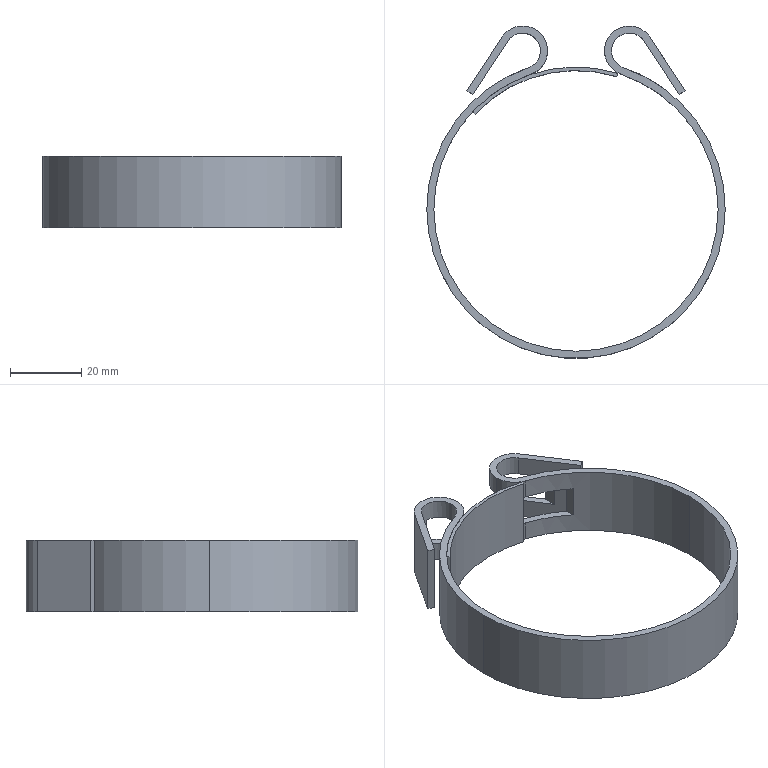Part | SolidWorks | features ICE 3, Extrusion 1 | 2 solids | 38 faces | box 84 x 93.542 x 20 mm | volume 12226 mm3 | plane 20 | cylinder 18 | commonest cylinder face diameters 10 x5 14 x5 80 x4 84 x3 78 x1
STEP:
#1=CARTESIAN_POINT('',(12.766,37.908,5.5));
#2=VERTEX_POINT('',#1);
#3=CARTESIAN_POINT('',(8.,44.542,5.5));
#4=VERTEX_POINT('',#3);
#5=CARTESIAN_POINT('',(15.,44.542,5.5));
#6=DIRECTION('',(0.,0.,-1.));
#7=DIRECTION('',(-1.,0.,0.));
#8=AXIS2_PLACEMENT_3D('',#5,#6,#7);
#9=CIRCLE('',#8,7.);
#10=EDGE_CURVE('',#2,#4,#9,.T.);
#11=ORIENTED_EDGE('',*,*,#10,.T.);
#12=CARTESIAN_POINT('',(8.,44.542,0.));
#13=VERTEX_POINT('',#12);
#14=CARTESIAN_POINT('',(8.,44.542,20.));
#15=DIRECTION('',(0.,0.,-1.));
#16=VECTOR('',#15,1000.);
#17=LINE('',#14,#16);
#18=EDGE_CURVE('',#4,#13,#17,.T.);
#19=ORIENTED_EDGE('',*,*,#18,.T.);
#20=CARTESIAN_POINT('',(12.766,37.908,0.));
#21=VERTEX_POINT('',#20);
#22=CARTESIAN_POINT('',(15.,44.542,0.));
#23=DIRECTION('',(0.,0.,1.));
#24=DIRECTION('',(-1.,0.,0.));
#25=AXIS2_PLACEMENT_3D('',#22,#23,#24);
#26=CIRCLE('',#25,7.);
#27=EDGE_CURVE('',#13,#21,#26,.T.);
#28=ORIENTED_EDGE('',*,*,#27,.T.);
#29=CARTESIAN_POINT('',(12.766,37.908,20.));
#30=DIRECTION('',(0.,0.,-1.));
#31=VECTOR('',#30,1000.);
#32=LINE('',#29,#31);
#33=EDGE_CURVE('',#2,#21,#32,.T.);
#34=ORIENTED_EDGE('',*,*,#33,.F.);
#35=EDGE_LOOP('',(#11,#19,#28,#34));
#36=FACE_OUTER_BOUND('',#35,.T.);
#37=CARTESIAN_POINT('',(15.,44.542,20.));
#38=DIRECTION('',(0.,0.,-1.));
#39=DIRECTION('',(-1.,0.,0.));
#40=AXIS2_PLACEMENT_3D('',#37,#38,#39);
#41=CYLINDRICAL_SURFACE('',#40,7.);
#42=ADVANCED_FACE('',(#36),#41,.T.);
#43=CARTESIAN_POINT('',(10.,44.542,20.));
#44=VERTEX_POINT('',#43);
#45=CARTESIAN_POINT('',(19.178,47.288,20.));
#46=VERTEX_POINT('',#45);
#47=CARTESIAN_POINT('',(15.,44.542,20.));
#48=DIRECTION('',(0.,0.,-1.));
#49=DIRECTION('',(-1.,0.,0.));
#50=AXIS2_PLACEMENT_3D('',#47,#48,#49);
#51=CIRCLE('',#50,5.);
#52=EDGE_CURVE('',#44,#46,#51,.T.);
#53=ORIENTED_EDGE('',*,*,#52,.F.);
#54=CARTESIAN_POINT('',(10.,44.542,14.5));
#55=VERTEX_POINT('',#54);
#56=CARTESIAN_POINT('',(10.,44.542,20.));
#57=DIRECTION('',(0.,0.,-1.));
#58=VECTOR('',#57,1000.);
#59=LINE('',#56,#58);
#60=EDGE_CURVE('',#44,#55,#59,.T.);
#61=ORIENTED_EDGE('',*,*,#60,.T.);
#62=CARTESIAN_POINT('',(19.178,47.288,14.5));
#63=VERTEX_POINT('',#62);
#64=CARTESIAN_POINT('',(15.,44.542,14.5));
#65=DIRECTION('',(0.,0.,-1.));
#66=DIRECTION('',(1.,0.,0.));
#67=AXIS2_PLACEMENT_3D('',#64,#65,#66);
#68=CIRCLE('',#67,5.);
#69=EDGE_CURVE('',#55,#63,#68,.T.);
#70=ORIENTED_EDGE('',*,*,#69,.T.);
#71=CARTESIAN_POINT('',(19.178,47.288,20.));
#72=DIRECTION('',(0.,0.,-1.));
#73=VECTOR('',#72,1000.);
#74=LINE('',#71,#73);
#75=EDGE_CURVE('',#46,#63,#74,.T.);
#76=ORIENTED_EDGE('',*,*,#75,.F.);
#77=EDGE_LOOP('',(#53,#61,#70,#76));
#78=FACE_OUTER_BOUND('',#77,.T.);
#79=CARTESIAN_POINT('',(15.,44.542,20.));
#80=DIRECTION('',(0.,0.,-1.));
#81=DIRECTION('',(-1.,0.,0.));
#82=AXIS2_PLACEMENT_3D('',#79,#80,#81);
#83=CYLINDRICAL_SURFACE('',#82,5.);
#84=ADVANCED_FACE('',(#78),#83,.F.);
#85=CARTESIAN_POINT('',(40.,0.,20.));
#86=VERTEX_POINT('',#85);
#87=CARTESIAN_POINT('',(-40.,0.,20.));
#88=VERTEX_POINT('',#87);
#89=CARTESIAN_POINT('',(0.,0.,20.));
#90=DIRECTION('',(0.,0.,-1.));
#91=DIRECTION('',(1.,0.,0.));
#92=AXIS2_PLACEMENT_3D('',#89,#90,#91);
#93=CIRCLE('',#92,40.);
#94=EDGE_CURVE('',#86,#88,#93,.T.);
#95=ORIENTED_EDGE('',*,*,#94,.F.);
#96=CARTESIAN_POINT('',(40.,0.,0.));
#97=VERTEX_POINT('',#96);
#98=CARTESIAN_POINT('',(40.,0.,20.));
#99=DIRECTION('',(0.,0.,-1.));
#100=VECTOR('',#99,1000.);
#101=LINE('',#98,#100);
#102=EDGE_CURVE('',#86,#97,#101,.T.);
#103=ORIENTED_EDGE('',*,*,#102,.T.);
#104=CARTESIAN_POINT('',(-40.,0.,0.));
#105=VERTEX_POINT('',#104);
#106=CARTESIAN_POINT('',(0.,0.,0.));
#107=DIRECTION('',(0.,0.,-1.));
#108=DIRECTION('',(1.,0.,0.));
#109=AXIS2_PLACEMENT_3D('',#106,#107,#108);
#110=CIRCLE('',#109,40.);
#111=EDGE_CURVE('',#97,#105,#110,.T.);
#112=ORIENTED_EDGE('',*,*,#111,.T.);
#113=CARTESIAN_POINT('',(-40.,0.,20.));
#114=DIRECTION('',(0.,0.,-1.));
#115=VECTOR('',#114,1000.);
#116=LINE('',#113,#115);
#117=EDGE_CURVE('',#88,#105,#116,.T.);
#118=ORIENTED_EDGE('',*,*,#117,.F.);
#119=EDGE_LOOP('',(#95,#103,#112,#118));
#120=FACE_OUTER_BOUND('',#119,.T.);
#121=CARTESIAN_POINT('',(0.,0.,20.));
#122=DIRECTION('',(0.,0.,-1.));
#123=DIRECTION('',(-1.,0.,0.));
#124=AXIS2_PLACEMENT_3D('',#121,#122,#123);
#125=CYLINDRICAL_SURFACE('',#124,40.);
#126=ADVANCED_FACE('',(#120),#125,.F.);
#127=CARTESIAN_POINT('',(-12.766,37.908,20.));
#128=VERTEX_POINT('',#127);
#129=CARTESIAN_POINT('',(0.,0.,20.));
#130=DIRECTION('',(0.,0.,-1.));
#131=DIRECTION('',(1.,0.,0.));
#132=AXIS2_PLACEMENT_3D('',#129,#130,#131);
#133=CIRCLE('',#132,40.);
#134=EDGE_CURVE('',#88,#128,#133,.T.);
#135=ORIENTED_EDGE('',*,*,#134,.F.);
#136=ORIENTED_EDGE('',*,*,#117,.T.);
#137=CARTESIAN_POINT('',(-12.766,37.908,0.));
#138=VERTEX_POINT('',#137);
#139=CARTESIAN_POINT('',(0.,0.,0.));
#140=DIRECTION('',(0.,0.,-1.));
#141=DIRECTION('',(1.,0.,0.));
#142=AXIS2_PLACEMENT_3D('',#139,#140,#141);
#143=CIRCLE('',#142,40.);
#144=EDGE_CURVE('',#105,#138,#143,.T.);
#145=ORIENTED_EDGE('',*,*,#144,.T.);
#146=CARTESIAN_POINT('',(-12.766,37.908,5.5));
#147=VERTEX_POINT('',#146);
#148=CARTESIAN_POINT('',(-12.766,37.908,20.));
#149=DIRECTION('',(0.,0.,-1.));
#150=VECTOR('',#149,1000.);
#151=LINE('',#148,#150);
#152=EDGE_CURVE('',#147,#138,#151,.T.);
#153=ORIENTED_EDGE('',*,*,#152,.F.);
#154=CARTESIAN_POINT('',(-15.,37.081,5.5));
#155=VERTEX_POINT('',#154);
#156=CARTESIAN_POINT('',(0.,0.,5.5));
#157=DIRECTION('',(0.,0.,-1.));
#158=DIRECTION('',(1.,0.,0.));
#159=AXIS2_PLACEMENT_3D('',#156,#157,#158);
#160=CIRCLE('',#159,40.);
#161=EDGE_CURVE('',#155,#147,#160,.T.);
#162=ORIENTED_EDGE('',*,*,#161,.F.);
#163=CARTESIAN_POINT('',(-15.,37.081,14.5));
#164=VERTEX_POINT('',#163);
#165=CARTESIAN_POINT('',(-15.,37.081,20.));
#166=DIRECTION('',(0.,0.,-1.));
#167=VECTOR('',#166,1000.);
#168=LINE('',#165,#167);
#169=EDGE_CURVE('',#164,#155,#168,.T.);
#170=ORIENTED_EDGE('',*,*,#169,.F.);
#171=CARTESIAN_POINT('',(-12.766,37.908,14.5));
#172=VERTEX_POINT('',#171);
#173=CARTESIAN_POINT('',(0.,0.,14.5));
#174=DIRECTION('',(0.,0.,1.));
#175=DIRECTION('',(-1.,0.,0.));
#176=AXIS2_PLACEMENT_3D('',#173,#174,#175);
#177=CIRCLE('',#176,40.);
#178=EDGE_CURVE('',#172,#164,#177,.T.);
#179=ORIENTED_EDGE('',*,*,#178,.F.);
#180=CARTESIAN_POINT('',(-12.766,37.908,20.));
#181=DIRECTION('',(0.,0.,-1.));
#182=VECTOR('',#181,1000.);
#183=LINE('',#180,#182);
#184=EDGE_CURVE('',#128,#172,#183,.T.);
#185=ORIENTED_EDGE('',*,*,#184,.F.);
#186=EDGE_LOOP('',(#135,#136,#145,#153,#162,#170,#179,#185));
#187=FACE_OUTER_BOUND('',#186,.T.);
#188=CARTESIAN_POINT('',(0.,0.,20.));
#189=DIRECTION('',(0.,0.,-1.));
#190=DIRECTION('',(-1.,0.,0.));
#191=AXIS2_PLACEMENT_3D('',#188,#189,#190);
#192=CYLINDRICAL_SURFACE('',#191,40.);
#193=ADVANCED_FACE('',(#187),#192,.F.);
#194=CARTESIAN_POINT('',(42.,0.,20.));
#195=VERTEX_POINT('',#194);
#196=CARTESIAN_POINT('',(13.404,39.804,20.));
#197=VERTEX_POINT('',#196);
#198=CARTESIAN_POINT('',(0.,0.,20.));
#199=DIRECTION('',(0.,0.,1.));
#200=DIRECTION('',(1.,0.,0.));
#201=AXIS2_PLACEMENT_3D('',#198,#199,#200);
#202=CIRCLE('',#201,42.);
#203=EDGE_CURVE('',#195,#197,#202,.T.);
#204=ORIENTED_EDGE('',*,*,#203,.F.);
#205=CARTESIAN_POINT('',(42.,0.,0.));
#206=VERTEX_POINT('',#205);
#207=CARTESIAN_POINT('',(42.,0.,20.));
#208=DIRECTION('',(0.,0.,-1.));
#209=VECTOR('',#208,1000.);
#210=LINE('',#207,#209);
#211=EDGE_CURVE('',#195,#206,#210,.T.);
#212=ORIENTED_EDGE('',*,*,#211,.T.);
#213=CARTESIAN_POINT('',(13.404,39.804,0.));
#214=VERTEX_POINT('',#213);
#215=CARTESIAN_POINT('',(0.,0.,0.));
#216=DIRECTION('',(0.,0.,1.));
#217=DIRECTION('',(1.,0.,0.));
#218=AXIS2_PLACEMENT_3D('',#215,#216,#217);
#219=CIRCLE('',#218,42.);
#220=EDGE_CURVE('',#206,#214,#219,.T.);
#221=ORIENTED_EDGE('',*,*,#220,.T.);
#222=CARTESIAN_POINT('',(13.404,39.804,5.5));
#223=VERTEX_POINT('',#222);
#224=CARTESIAN_POINT('',(13.404,39.804,20.));
#225=DIRECTION('',(0.,0.,-1.));
#226=VECTOR('',#225,1000.);
#227=LINE('',#224,#226);
#228=EDGE_CURVE('',#223,#214,#227,.T.);
#229=ORIENTED_EDGE('',*,*,#228,.F.);
#230=CARTESIAN_POINT('',(25.,33.749,5.5));
#231=VERTEX_POINT('',#230);
#232=CARTESIAN_POINT('',(0.,0.,5.5));
#233=DIRECTION('',(0.,0.,-1.));
#234=DIRECTION('',(-1.,0.,0.));
#235=AXIS2_PLACEMENT_3D('',#232,#233,#234);
#236=CIRCLE('',#235,42.);
#237=EDGE_CURVE('',#223,#231,#236,.T.);
#238=ORIENTED_EDGE('',*,*,#237,.T.);
#239=CARTESIAN_POINT('',(25.,33.749,14.5));
#240=VERTEX_POINT('',#239);
#241=CARTESIAN_POINT('',(25.,33.749,20.));
#242=DIRECTION('',(0.,0.,1.));
#243=VECTOR('',#242,1000.);
#244=LINE('',#241,#243);
#245=EDGE_CURVE('',#231,#240,#244,.T.);
#246=ORIENTED_EDGE('',*,*,#245,.T.);
#247=CARTESIAN_POINT('',(13.404,39.804,14.5));
#248=VERTEX_POINT('',#247);
#249=CARTESIAN_POINT('',(0.,0.,14.5));
#250=DIRECTION('',(0.,0.,1.));
#251=DIRECTION('',(1.,0.,0.));
#252=AXIS2_PLACEMENT_3D('',#249,#250,#251);
#253=CIRCLE('',#252,42.);
#254=EDGE_CURVE('',#240,#248,#253,.T.);
#255=ORIENTED_EDGE('',*,*,#254,.T.);
#256=CARTESIAN_POINT('',(13.404,39.804,20.));
#257=DIRECTION('',(0.,0.,-1.));
#258=VECTOR('',#257,1000.);
#259=LINE('',#256,#258);
#260=EDGE_CURVE('',#197,#248,#259,.T.);
#261=ORIENTED_EDGE('',*,*,#260,.F.);
#262=EDGE_LOOP('',(#204,#212,#221,#229,#238,#246,#255,#261));
#263=FACE_OUTER_BOUND('',#262,.T.);
#264=CARTESIAN_POINT('',(0.,0.,20.));
#265=DIRECTION('',(0.,0.,-1.));
#266=DIRECTION('',(-1.,0.,0.));
#267=AXIS2_PLACEMENT_3D('',#264,#265,#266);
#268=CYLINDRICAL_SURFACE('',#267,42.);
#269=ADVANCED_FACE('',(#263),#268,.T.);
#270=ORIENTED_EDGE('',*,*,#211,.F.);
#271=CARTESIAN_POINT('',(-42.,0.,20.));
#272=VERTEX_POINT('',#271);
#273=CARTESIAN_POINT('',(0.,0.,20.));
#274=DIRECTION('',(0.,0.,1.));
#275=DIRECTION('',(1.,0.,0.));
#276=AXIS2_PLACEMENT_3D('',#273,#274,#275);
#277=CIRCLE('',#276,42.);
#278=EDGE_CURVE('',#272,#195,#277,.T.);
#279=ORIENTED_EDGE('',*,*,#278,.F.);
#280=CARTESIAN_POINT('',(-42.,0.,0.));
#281=VERTEX_POINT('',#280);
#282=CARTESIAN_POINT('',(-42.,0.,20.));
#283=DIRECTION('',(0.,0.,-1.));
#284=VECTOR('',#283,1000.);
#285=LINE('',#282,#284);
#286=EDGE_CURVE('',#272,#281,#285,.T.);
#287=ORIENTED_EDGE('',*,*,#286,.T.);
#288=CARTESIAN_POINT('',(0.,0.,0.));
#289=DIRECTION('',(0.,0.,1.));
#290=DIRECTION('',(1.,0.,0.));
#291=AXIS2_PLACEMENT_3D('',#288,#289,#290);
#292=CIRCLE('',#291,42.);
#293=EDGE_CURVE('',#281,#206,#292,.T.);
#294=ORIENTED_EDGE('',*,*,#293,.T.);
#295=EDGE_LOOP('',(#270,#279,#287,#294));
#296=FACE_OUTER_BOUND('',#295,.T.);
#297=CARTESIAN_POINT('',(0.,0.,20.));
#298=DIRECTION('',(0.,0.,-1.));
#299=DIRECTION('',(-1.,0.,0.));
#300=AXIS2_PLACEMENT_3D('',#297,#298,#299);
#301=CYLINDRICAL_SURFACE('',#300,42.);
#302=ADVANCED_FACE('',(#296),#301,.T.);
#303=CARTESIAN_POINT('',(8.,44.542,20.));
#304=VERTEX_POINT('',#303);
#305=CARTESIAN_POINT('',(12.766,37.908,20.));
#306=VERTEX_POINT('',#305);
#307=CARTESIAN_POINT('',(15.,44.542,20.));
#308=DIRECTION('',(0.,0.,1.));
#309=DIRECTION('',(-1.,0.,0.));
#310=AXIS2_PLACEMENT_3D('',#307,#308,#309);
#311=CIRCLE('',#310,7.);
#312=EDGE_CURVE('',#304,#306,#311,.T.);
#313=ORIENTED_EDGE('',*,*,#312,.F.);
#314=CARTESIAN_POINT('',(8.,44.542,14.5));
#315=VERTEX_POINT('',#314);
#316=CARTESIAN_POINT('',(8.,44.542,20.));
#317=DIRECTION('',(0.,0.,-1.));
#318=VECTOR('',#317,1000.);
#319=LINE('',#316,#318);
#320=EDGE_CURVE('',#304,#315,#319,.T.);
#321=ORIENTED_EDGE('',*,*,#320,.T.);
#322=CARTESIAN_POINT('',(12.766,37.908,14.5));
#323=VERTEX_POINT('',#322);
#324=CARTESIAN_POINT('',(15.,44.542,14.5));
#325=DIRECTION('',(0.,0.,1.));
#326=DIRECTION('',(1.,0.,0.));
#327=AXIS2_PLACEMENT_3D('',#324,#325,#326);
#328=CIRCLE('',#327,7.);
#329=EDGE_CURVE('',#315,#323,#328,.T.);
#330=ORIENTED_EDGE('',*,*,#329,.T.);
#331=CARTESIAN_POINT('',(12.766,37.908,20.));
#332=DIRECTION('',(0.,0.,-1.));
#333=VECTOR('',#332,1000.);
#334=LINE('',#331,#333);
#335=EDGE_CURVE('',#306,#323,#334,.T.);
#336=ORIENTED_EDGE('',*,*,#335,.F.);
#337=EDGE_LOOP('',(#313,#321,#330,#336));
#338=FACE_OUTER_BOUND('',#337,.T.);
#339=CARTESIAN_POINT('',(15.,44.542,20.));
#340=DIRECTION('',(0.,0.,-1.));
#341=DIRECTION('',(-1.,0.,0.));
#342=AXIS2_PLACEMENT_3D('',#339,#340,#341);
#343=CYLINDRICAL_SURFACE('',#342,7.);
#344=ADVANCED_FACE('',(#338),#343,.T.);
#345=CARTESIAN_POINT('',(19.178,47.288,5.5));
#346=VERTEX_POINT('',#345);
#347=CARTESIAN_POINT('',(10.,44.542,5.5));
#348=VERTEX_POINT('',#347);
#349=CARTESIAN_POINT('',(15.,44.542,5.5));
#350=DIRECTION('',(0.,0.,1.));
#351=DIRECTION('',(-1.,0.,0.));
#352=AXIS2_PLACEMENT_3D('',#349,#350,#351);
#353=CIRCLE('',#352,5.);
#354=EDGE_CURVE('',#346,#348,#353,.T.);
#355=ORIENTED_EDGE('',*,*,#354,.T.);
#356=CARTESIAN_POINT('',(10.,44.542,0.));
#357=VERTEX_POINT('',#356);
#358=CARTESIAN_POINT('',(10.,44.542,20.));
#359=DIRECTION('',(0.,0.,-1.));
#360=VECTOR('',#359,1000.);
#361=LINE('',#358,#360);
#362=EDGE_CURVE('',#348,#357,#361,.T.);
#363=ORIENTED_EDGE('',*,*,#362,.T.);
#364=CARTESIAN_POINT('',(19.178,47.288,0.));
#365=VERTEX_POINT('',#364);
#366=CARTESIAN_POINT('',(15.,44.542,0.));
#367=DIRECTION('',(0.,0.,-1.));
#368=DIRECTION('',(-1.,0.,0.));
#369=AXIS2_PLACEMENT_3D('',#366,#367,#368);
#370=CIRCLE('',#369,5.);
#371=EDGE_CURVE('',#357,#365,#370,.T.);
#372=ORIENTED_EDGE('',*,*,#371,.T.);
#373=CARTESIAN_POINT('',(19.178,47.288,20.));
#374=DIRECTION('',(0.,0.,-1.));
#375=VECTOR('',#374,1000.);
#376=LINE('',#373,#375);
#377=EDGE_CURVE('',#346,#365,#376,.T.);
#378=ORIENTED_EDGE('',*,*,#377,.F.);
#379=EDGE_LOOP('',(#355,#363,#372,#378));
#380=FACE_OUTER_BOUND('',#379,.T.);
#381=CARTESIAN_POINT('',(15.,44.542,20.));
#382=DIRECTION('',(0.,0.,-1.));
#383=DIRECTION('',(-1.,0.,0.));
#384=AXIS2_PLACEMENT_3D('',#381,#382,#383);
#385=CYLINDRICAL_SURFACE('',#384,5.);
#386=ADVANCED_FACE('',(#380),#385,.F.);
#387=ORIENTED_EDGE('',*,*,#362,.F.);
#388=CARTESIAN_POINT('',(15.,44.542,5.5));
#389=DIRECTION('',(0.,0.,1.));
#390=DIRECTION('',(-1.,0.,0.));
#391=AXIS2_PLACEMENT_3D('',#388,#389,#390);
#392=CIRCLE('',#391,5.);
#393=EDGE_CURVE('',#348,#223,#392,.T.);
#394=ORIENTED_EDGE('',*,*,#393,.T.);
#395=ORIENTED_EDGE('',*,*,#228,.T.);
#396=CARTESIAN_POINT('',(15.,44.542,0.));
#397=DIRECTION('',(0.,0.,-1.));
#398=DIRECTION('',(-1.,0.,0.));
#399=AXIS2_PLACEMENT_3D('',#396,#397,#398);
#400=CIRCLE('',#399,5.);
#401=EDGE_CURVE('',#214,#357,#400,.T.);
#402=ORIENTED_EDGE('',*,*,#401,.T.);
#403=EDGE_LOOP('',(#387,#394,#395,#402));
#404=FACE_OUTER_BOUND('',#403,.T.);
#405=CARTESIAN_POINT('',(15.,44.542,20.));
#406=DIRECTION('',(0.,0.,-1.));
#407=DIRECTION('',(-1.,0.,0.));
#408=AXIS2_PLACEMENT_3D('',#405,#406,#407);
#409=CYLINDRICAL_SURFACE('',#408,5.);
#410=ADVANCED_FACE('',(#404),#409,.F.);
#411=ORIENTED_EDGE('',*,*,#320,.F.);
#412=CARTESIAN_POINT('',(20.85,48.387,20.));
#413=VERTEX_POINT('',#412);
#414=CARTESIAN_POINT('',(15.,44.542,20.));
#415=DIRECTION('',(0.,0.,1.));
#416=DIRECTION('',(-1.,0.,0.));
#417=AXIS2_PLACEMENT_3D('',#414,#415,#416);
#418=CIRCLE('',#417,7.);
#419=EDGE_CURVE('',#413,#304,#418,.T.);
#420=ORIENTED_EDGE('',*,*,#419,.F.);
#421=CARTESIAN_POINT('',(20.85,48.387,14.5));
#422=VERTEX_POINT('',#421);
#423=CARTESIAN_POINT('',(20.85,48.387,20.));
#424=DIRECTION('',(0.,0.,-1.));
#425=VECTOR('',#424,1000.);
#426=LINE('',#423,#425);
#427=EDGE_CURVE('',#413,#422,#426,.T.);
#428=ORIENTED_EDGE('',*,*,#427,.T.);
#429=CARTESIAN_POINT('',(15.,44.542,14.5));
#430=DIRECTION('',(0.,0.,1.));
#431=DIRECTION('',(1.,0.,0.));
#432=AXIS2_PLACEMENT_3D('',#429,#430,#431);
#433=CIRCLE('',#432,7.);
#434=EDGE_CURVE('',#422,#315,#433,.T.);
#435=ORIENTED_EDGE('',*,*,#434,.T.);
#436=EDGE_LOOP('',(#411,#420,#428,#435));
#437=FACE_OUTER_BOUND('',#436,.T.);
#438=CARTESIAN_POINT('',(15.,44.542,20.));
#439=DIRECTION('',(0.,0.,-1.));
#440=DIRECTION('',(-1.,0.,0.));
#441=AXIS2_PLACEMENT_3D('',#438,#439,#440);
#442=CYLINDRICAL_SURFACE('',#441,7.);
#443=ADVANCED_FACE('',(#437),#442,.T.);
#444=CARTESIAN_POINT('',(-15.,49.542,5.5));
#445=VERTEX_POINT('',#444);
#446=CARTESIAN_POINT('',(-13.404,39.804,5.5));
#447=VERTEX_POINT('',#446);
#448=CARTESIAN_POINT('',(-15.,44.542,5.5));
#449=DIRECTION('',(0.,0.,-1.));
#450=DIRECTION('',(1.,0.,0.));
#451=AXIS2_PLACEMENT_3D('',#448,#449,#450);
#452=CIRCLE('',#451,5.);
#453=EDGE_CURVE('',#445,#447,#452,.T.);
#454=ORIENTED_EDGE('',*,*,#453,.F.);
#455=CARTESIAN_POINT('',(-15.,49.542,14.5));
#456=VERTEX_POINT('',#455);
#457=CARTESIAN_POINT('',(-15.,49.542,20.));
#458=DIRECTION('',(0.,0.,-1.));
#459=VECTOR('',#458,1000.);
#460=LINE('',#457,#459);
#461=EDGE_CURVE('',#456,#445,#460,.T.);
#462=ORIENTED_EDGE('',*,*,#461,.F.);
#463=CARTESIAN_POINT('',(-13.404,39.804,14.5));
#464=VERTEX_POINT('',#463);
#465=CARTESIAN_POINT('',(-15.,44.542,14.5));
#466=DIRECTION('',(0.,0.,1.));
#467=DIRECTION('',(-1.,0.,0.));
#468=AXIS2_PLACEMENT_3D('',#465,#466,#467);
#469=CIRCLE('',#468,5.);
#470=EDGE_CURVE('',#464,#456,#469,.T.);
#471=ORIENTED_EDGE('',*,*,#470,.F.);
#472=CARTESIAN_POINT('',(-13.404,39.804,20.));
#473=VERTEX_POINT('',#472);
#474=CARTESIAN_POINT('',(-13.404,39.804,20.));
#475=DIRECTION('',(0.,0.,-1.));
#476=VECTOR('',#475,1000.);
#477=LINE('',#474,#476);
#478=EDGE_CURVE('',#473,#464,#477,.T.);
#479=ORIENTED_EDGE('',*,*,#478,.F.);
#480=CARTESIAN_POINT('',(-19.178,47.288,20.));
#481=VERTEX_POINT('',#480);
#482=CARTESIAN_POINT('',(-15.,44.542,20.));
#483=DIRECTION('',(0.,0.,-1.));
#484=DIRECTION('',(1.,0.,0.));
#485=AXIS2_PLACEMENT_3D('',#482,#483,#484);
#486=CIRCLE('',#485,5.);
#487=EDGE_CURVE('',#481,#473,#486,.T.);
#488=ORIENTED_EDGE('',*,*,#487,.F.);
#489=CARTESIAN_POINT('',(-19.178,47.288,0.));
#490=VERTEX_POINT('',#489);
#491=CARTESIAN_POINT('',(-19.178,47.288,20.));
#492=DIRECTION('',(0.,0.,-1.));
#493=VECTOR('',#492,1000.);
#494=LINE('',#491,#493);
#495=EDGE_CURVE('',#481,#490,#494,.T.);
#496=ORIENTED_EDGE('',*,*,#495,.T.);
#497=CARTESIAN_POINT('',(-13.404,39.804,0.));
#498=VERTEX_POINT('',#497);
#499=CARTESIAN_POINT('',(-15.,44.542,0.));
#500=DIRECTION('',(0.,0.,-1.));
#501=DIRECTION('',(1.,0.,0.));
#502=AXIS2_PLACEMENT_3D('',#499,#500,#501);
#503=CIRCLE('',#502,5.);
#504=EDGE_CURVE('',#490,#498,#503,.T.);
#505=ORIENTED_EDGE('',*,*,#504,.T.);
#506=CARTESIAN_POINT('',(-13.404,39.804,20.));
#507=DIRECTION('',(0.,0.,-1.));
#508=VECTOR('',#507,1000.);
#509=LINE('',#506,#508);
#510=EDGE_CURVE('',#447,#498,#509,.T.);
#511=ORIENTED_EDGE('',*,*,#510,.F.);
#512=EDGE_LOOP('',(#454,#462,#471,#479,#488,#496,#505,#511));
#513=FACE_OUTER_BOUND('',#512,.T.);
#514=CARTESIAN_POINT('',(-15.,44.542,20.));
#515=DIRECTION('',(0.,0.,-1.));
#516=DIRECTION('',(-1.,0.,0.));
#517=AXIS2_PLACEMENT_3D('',#514,#515,#516);
#518=CYLINDRICAL_SURFACE('',#517,5.);
#519=ADVANCED_FACE('',(#513),#518,.F.);
#520=ORIENTED_EDGE('',*,*,#286,.F.);
#521=CARTESIAN_POINT('',(0.,0.,20.));
#522=DIRECTION('',(0.,0.,1.));
#523=DIRECTION('',(1.,0.,0.));
#524=AXIS2_PLACEMENT_3D('',#521,#522,#523);
#525=CIRCLE('',#524,42.);
#526=EDGE_CURVE('',#473,#272,#525,.T.);
#527=ORIENTED_EDGE('',*,*,#526,.F.);
#528=ORIENTED_EDGE('',*,*,#478,.T.);
#529=CARTESIAN_POINT('',(-15.,39.23,14.5));
#530=VERTEX_POINT('',#529);
#531=CARTESIAN_POINT('',(0.,0.,14.5));
#532=DIRECTION('',(0.,0.,-1.));
#533=DIRECTION('',(-1.,0.,0.));
#534=AXIS2_PLACEMENT_3D('',#531,#532,#533);
#535=CIRCLE('',#534,42.);
#536=EDGE_CURVE('',#530,#464,#535,.T.);
#537=ORIENTED_EDGE('',*,*,#536,.F.);
#538=CARTESIAN_POINT('',(-15.,39.23,5.5));
#539=VERTEX_POINT('',#538);
#540=CARTESIAN_POINT('',(-15.,39.23,20.));
#541=DIRECTION('',(0.,0.,1.));
#542=VECTOR('',#541,1000.);
#543=LINE('',#540,#542);
#544=EDGE_CURVE('',#539,#530,#543,.T.);
#545=ORIENTED_EDGE('',*,*,#544,.F.);
#546=CARTESIAN_POINT('',(0.,0.,5.5));
#547=DIRECTION('',(0.,0.,1.));
#548=DIRECTION('',(1.,0.,0.));
#549=AXIS2_PLACEMENT_3D('',#546,#547,#548);
#550=CIRCLE('',#549,42.);
#551=EDGE_CURVE('',#447,#539,#550,.T.);
#552=ORIENTED_EDGE('',*,*,#551,.F.);
#553=ORIENTED_EDGE('',*,*,#510,.T.);
#554=CARTESIAN_POINT('',(0.,0.,0.));
#555=DIRECTION('',(0.,0.,1.));
#556=DIRECTION('',(1.,0.,0.));
#557=AXIS2_PLACEMENT_3D('',#554,#555,#556);
#558=CIRCLE('',#557,42.);
#559=EDGE_CURVE('',#498,#281,#558,.T.);
#560=ORIENTED_EDGE('',*,*,#559,.T.);
#561=EDGE_LOOP('',(#520,#527,#528,#537,#545,#552,#553,#560));
#562=FACE_OUTER_BOUND('',#561,.T.);
#563=CARTESIAN_POINT('',(0.,0.,20.));
#564=DIRECTION('',(0.,0.,-1.));
#565=DIRECTION('',(-1.,0.,0.));
#566=AXIS2_PLACEMENT_3D('',#563,#564,#565);
#567=CYLINDRICAL_SURFACE('',#566,42.);
#568=ADVANCED_FACE('',(#562),#567,.T.);
#569=ORIENTED_EDGE('',*,*,#102,.F.);
#570=CARTESIAN_POINT('',(0.,0.,20.));
#571=DIRECTION('',(0.,0.,-1.));
#572=DIRECTION('',(1.,0.,0.));
#573=AXIS2_PLACEMENT_3D('',#570,#571,#572);
#574=CIRCLE('',#573,40.);
#575=EDGE_CURVE('',#306,#86,#574,.T.);
#576=ORIENTED_EDGE('',*,*,#575,.F.);
#577=ORIENTED_EDGE('',*,*,#335,.T.);
#578=CARTESIAN_POINT('',(25.,31.225,14.5));
#579=VERTEX_POINT('',#578);
#580=CARTESIAN_POINT('',(0.,0.,14.5));
#581=DIRECTION('',(0.,0.,-1.));
#582=DIRECTION('',(1.,0.,0.));
#583=AXIS2_PLACEMENT_3D('',#580,#581,#582);
#584=CIRCLE('',#583,40.);
#585=EDGE_CURVE('',#323,#579,#584,.T.);
#586=ORIENTED_EDGE('',*,*,#585,.T.);
#587=CARTESIAN_POINT('',(25.,31.225,5.5));
#588=VERTEX_POINT('',#587);
#589=CARTESIAN_POINT('',(25.,31.225,20.));
#590=DIRECTION('',(0.,0.,-1.));
#591=VECTOR('',#590,1000.);
#592=LINE('',#589,#591);
#593=EDGE_CURVE('',#579,#588,#592,.T.);
#594=ORIENTED_EDGE('',*,*,#593,.T.);
#595=CARTESIAN_POINT('',(0.,0.,5.5));
#596=DIRECTION('',(0.,0.,1.));
#597=DIRECTION('',(-1.,0.,0.));
#598=AXIS2_PLACEMENT_3D('',#595,#596,#597);
#599=CIRCLE('',#598,40.);
#600=EDGE_CURVE('',#588,#2,#599,.T.);
#601=ORIENTED_EDGE('',*,*,#600,.T.);
#602=ORIENTED_EDGE('',*,*,#33,.T.);
#603=CARTESIAN_POINT('',(0.,0.,0.));
#604=DIRECTION('',(0.,0.,-1.));
#605=DIRECTION('',(1.,0.,0.));
#606=AXIS2_PLACEMENT_3D('',#603,#604,#605);
#607=CIRCLE('',#606,40.);
#608=EDGE_CURVE('',#21,#97,#607,.T.);
#609=ORIENTED_EDGE('',*,*,#608,.T.);
#610=EDGE_LOOP('',(#569,#576,#577,#586,#594,#601,#602,#609));
#611=FACE_OUTER_BOUND('',#610,.T.);
#612=CARTESIAN_POINT('',(0.,0.,20.));
#613=DIRECTION('',(0.,0.,-1.));
#614=DIRECTION('',(-1.,0.,0.));
#615=AXIS2_PLACEMENT_3D('',#612,#613,#614);
#616=CYLINDRICAL_SURFACE('',#615,40.);
#617=ADVANCED_FACE('',(#611),#616,.F.);
#618=CARTESIAN_POINT('',(-15.,51.542,5.5));
#619=VERTEX_POINT('',#618);
#620=CARTESIAN_POINT('',(-15.,44.542,5.5));
#621=DIRECTION('',(0.,0.,1.));
#622=DIRECTION('',(1.,0.,0.));
#623=AXIS2_PLACEMENT_3D('',#620,#621,#622);
#624=CIRCLE('',#623,7.);
#625=EDGE_CURVE('',#147,#619,#624,.T.);
#626=ORIENTED_EDGE('',*,*,#625,.F.);
#627=ORIENTED_EDGE('',*,*,#152,.T.);
#628=CARTESIAN_POINT('',(-20.85,48.387,0.));
#629=VERTEX_POINT('',#628);
#630=CARTESIAN_POINT('',(-15.,44.542,0.));
#631=DIRECTION('',(0.,0.,1.));
#632=DIRECTION('',(1.,0.,0.));
#633=AXIS2_PLACEMENT_3D('',#630,#631,#632);
#634=CIRCLE('',#633,7.);
#635=EDGE_CURVE('',#138,#629,#634,.T.);
#636=ORIENTED_EDGE('',*,*,#635,.T.);
#637=CARTESIAN_POINT('',(-20.85,48.387,20.));
#638=VERTEX_POINT('',#637);
#639=CARTESIAN_POINT('',(-20.85,48.387,20.));
#640=DIRECTION('',(0.,0.,-1.));
#641=VECTOR('',#640,1000.);
#642=LINE('',#639,#641);
#643=EDGE_CURVE('',#638,#629,#642,.T.);
#644=ORIENTED_EDGE('',*,*,#643,.F.);
#645=CARTESIAN_POINT('',(-15.,44.542,20.));
#646=DIRECTION('',(0.,0.,1.));
#647=DIRECTION('',(1.,0.,0.));
#648=AXIS2_PLACEMENT_3D('',#645,#646,#647);
#649=CIRCLE('',#648,7.);
#650=EDGE_CURVE('',#128,#638,#649,.T.);
#651=ORIENTED_EDGE('',*,*,#650,.F.);
#652=ORIENTED_EDGE('',*,*,#184,.T.);
#653=CARTESIAN_POINT('',(-15.,51.542,14.5));
#654=VERTEX_POINT('',#653);
#655=CARTESIAN_POINT('',(-15.,44.542,14.5));
#656=DIRECTION('',(0.,0.,-1.));
#657=DIRECTION('',(-1.,0.,0.));
#658=AXIS2_PLACEMENT_3D('',#655,#656,#657);
#659=CIRCLE('',#658,7.);
#660=EDGE_CURVE('',#654,#172,#659,.T.);
#661=ORIENTED_EDGE('',*,*,#660,.F.);
#662=CARTESIAN_POINT('',(-15.,51.542,20.));
#663=DIRECTION('',(0.,0.,1.));
#664=VECTOR('',#663,1000.);
#665=LINE('',#662,#664);
#666=EDGE_CURVE('',#619,#654,#665,.T.);
#667=ORIENTED_EDGE('',*,*,#666,.F.);
#668=EDGE_LOOP('',(#626,#627,#636,#644,#651,#652,#661,#667));
#669=FACE_OUTER_BOUND('',#668,.T.);
#670=CARTESIAN_POINT('',(-15.,44.542,20.));
#671=DIRECTION('',(0.,0.,-1.));
#672=DIRECTION('',(-1.,0.,0.));
#673=AXIS2_PLACEMENT_3D('',#670,#671,#672);
#674=CYLINDRICAL_SURFACE('',#673,7.);
#675=ADVANCED_FACE('',(#669),#674,.T.);
#676=ORIENTED_EDGE('',*,*,#60,.F.);
#677=CARTESIAN_POINT('',(15.,44.542,20.));
#678=DIRECTION('',(0.,0.,-1.));
#679=DIRECTION('',(-1.,0.,0.));
#680=AXIS2_PLACEMENT_3D('',#677,#678,#679);
#681=CIRCLE('',#680,5.);
#682=EDGE_CURVE('',#197,#44,#681,.T.);
#683=ORIENTED_EDGE('',*,*,#682,.F.);
#684=ORIENTED_EDGE('',*,*,#260,.T.);
#685=CARTESIAN_POINT('',(15.,44.542,14.5));
#686=DIRECTION('',(0.,0.,-1.));
#687=DIRECTION('',(1.,0.,0.));
#688=AXIS2_PLACEMENT_3D('',#685,#686,#687);
#689=CIRCLE('',#688,5.);
#690=EDGE_CURVE('',#248,#55,#689,.T.);
#691=ORIENTED_EDGE('',*,*,#690,.T.);
#692=EDGE_LOOP('',(#676,#683,#684,#691));
#693=FACE_OUTER_BOUND('',#692,.T.);
#694=CARTESIAN_POINT('',(15.,44.542,20.));
#695=DIRECTION('',(0.,0.,-1.));
#696=DIRECTION('',(-1.,0.,0.));
#697=AXIS2_PLACEMENT_3D('',#694,#695,#696);
#698=CYLINDRICAL_SURFACE('',#697,5.);
#699=ADVANCED_FACE('',(#693),#698,.F.);
#700=CARTESIAN_POINT('',(25.,38.431,14.5));
#701=VERTEX_POINT('',#700);
#702=CARTESIAN_POINT('',(25.,38.431,5.5));
#703=VERTEX_POINT('',#702);
#704=CARTESIAN_POINT('',(25.,38.431,20.));
#705=DIRECTION('',(0.,0.,-1.));
#706=VECTOR('',#705,1000.);
#707=LINE('',#704,#706);
#708=EDGE_CURVE('',#701,#703,#707,.T.);
#709=ORIENTED_EDGE('',*,*,#708,.T.);
#710=CARTESIAN_POINT('',(19.178,47.288,5.5));
#711=DIRECTION('',(-0.5493,0.8357,0.));
#712=VECTOR('',#711,1000.);
#713=LINE('',#710,#712);
#714=EDGE_CURVE('',#703,#346,#713,.T.);
#715=ORIENTED_EDGE('',*,*,#714,.T.);
#716=ORIENTED_EDGE('',*,*,#377,.T.);
#717=CARTESIAN_POINT('',(29.065,32.247,0.));
#718=VERTEX_POINT('',#717);
#719=CARTESIAN_POINT('',(19.178,47.288,0.));
#720=DIRECTION('',(0.5493,-0.8357,0.));
#721=VECTOR('',#720,1000.);
#722=LINE('',#719,#721);
#723=EDGE_CURVE('',#365,#718,#722,.T.);
#724=ORIENTED_EDGE('',*,*,#723,.T.);
#725=CARTESIAN_POINT('',(29.065,32.247,20.));
#726=VERTEX_POINT('',#725);
#727=CARTESIAN_POINT('',(29.065,32.247,20.));
#728=DIRECTION('',(0.,0.,-1.));
#729=VECTOR('',#728,1000.);
#730=LINE('',#727,#729);
#731=EDGE_CURVE('',#726,#718,#730,.T.);
#732=ORIENTED_EDGE('',*,*,#731,.F.);
#733=CARTESIAN_POINT('',(19.178,47.288,20.));
#734=DIRECTION('',(0.5493,-0.8357,0.));
#735=VECTOR('',#734,1000.);
#736=LINE('',#733,#735);
#737=EDGE_CURVE('',#46,#726,#736,.T.);
#738=ORIENTED_EDGE('',*,*,#737,.F.);
#739=ORIENTED_EDGE('',*,*,#75,.T.);
#740=CARTESIAN_POINT('',(19.178,47.288,14.5));
#741=DIRECTION('',(0.5493,-0.8357,0.));
#742=VECTOR('',#741,1000.);
#743=LINE('',#740,#742);
#744=EDGE_CURVE('',#63,#701,#743,.T.);
#745=ORIENTED_EDGE('',*,*,#744,.T.);
#746=EDGE_LOOP('',(#709,#715,#716,#724,#732,#738,#739,#745));
#747=FACE_OUTER_BOUND('',#746,.T.);
#748=CARTESIAN_POINT('',(19.178,47.288,20.));
#749=DIRECTION('',(0.8357,0.5493,0.));
#750=DIRECTION('',(-0.5493,0.8357,0.));
#751=AXIS2_PLACEMENT_3D('',#748,#749,#750);
#752=PLANE('',#751);
#753=ADVANCED_FACE('',(#747),#752,.F.);
#754=CARTESIAN_POINT('',(30.736,33.345,0.));
#755=VERTEX_POINT('',#754);
#756=CARTESIAN_POINT('',(29.065,32.247,0.));
#757=DIRECTION('',(0.8357,0.5493,0.));
#758=VECTOR('',#757,1000.);
#759=LINE('',#756,#758);
#760=EDGE_CURVE('',#718,#755,#759,.T.);
#761=ORIENTED_EDGE('',*,*,#760,.T.);
#762=CARTESIAN_POINT('',(30.736,33.345,20.));
#763=VERTEX_POINT('',#762);
#764=CARTESIAN_POINT('',(30.736,33.345,20.));
#765=DIRECTION('',(0.,0.,-1.));
#766=VECTOR('',#765,1000.);
#767=LINE('',#764,#766);
#768=EDGE_CURVE('',#763,#755,#767,.T.);
#769=ORIENTED_EDGE('',*,*,#768,.F.);
#770=CARTESIAN_POINT('',(29.065,32.247,20.));
#771=DIRECTION('',(0.8357,0.5493,0.));
#772=VECTOR('',#771,1000.);
#773=LINE('',#770,#772);
#774=EDGE_CURVE('',#726,#763,#773,.T.);
#775=ORIENTED_EDGE('',*,*,#774,.F.);
#776=ORIENTED_EDGE('',*,*,#731,.T.);
#777=EDGE_LOOP('',(#761,#769,#775,#776));
#778=FACE_OUTER_BOUND('',#777,.T.);
#779=CARTESIAN_POINT('',(29.065,32.247,20.));
#780=DIRECTION('',(-0.5493,0.8357,0.));
#781=DIRECTION('',(-0.8357,-0.5493,0.));
#782=AXIS2_PLACEMENT_3D('',#779,#780,#781);
#783=PLANE('',#782);
#784=ADVANCED_FACE('',(#778),#783,.F.);
#785=CARTESIAN_POINT('',(20.85,48.387,5.5));
#786=VERTEX_POINT('',#785);
#787=CARTESIAN_POINT('',(20.85,48.387,0.));
#788=VERTEX_POINT('',#787);
#789=CARTESIAN_POINT('',(20.85,48.387,20.));
#790=DIRECTION('',(0.,0.,-1.));
#791=VECTOR('',#790,1000.);
#792=LINE('',#789,#791);
#793=EDGE_CURVE('',#786,#788,#792,.T.);
#794=ORIENTED_EDGE('',*,*,#793,.F.);
#795=CARTESIAN_POINT('',(25.,42.072,5.5));
#796=VERTEX_POINT('',#795);
#797=CARTESIAN_POINT('',(20.85,48.387,5.5));
#798=DIRECTION('',(0.5493,-0.8357,0.));
#799=VECTOR('',#798,1000.);
#800=LINE('',#797,#799);
#801=EDGE_CURVE('',#786,#796,#800,.T.);
#802=ORIENTED_EDGE('',*,*,#801,.T.);
#803=CARTESIAN_POINT('',(25.,42.072,14.5));
#804=VERTEX_POINT('',#803);
#805=CARTESIAN_POINT('',(25.,42.072,20.));
#806=DIRECTION('',(0.,0.,1.));
#807=VECTOR('',#806,1000.);
#808=LINE('',#805,#807);
#809=EDGE_CURVE('',#796,#804,#808,.T.);
#810=ORIENTED_EDGE('',*,*,#809,.T.);
#811=CARTESIAN_POINT('',(20.85,48.387,14.5));
#812=DIRECTION('',(-0.5493,0.8357,0.));
#813=VECTOR('',#812,1000.);
#814=LINE('',#811,#813);
#815=EDGE_CURVE('',#804,#422,#814,.T.);
#816=ORIENTED_EDGE('',*,*,#815,.T.);
#817=ORIENTED_EDGE('',*,*,#427,.F.);
#818=CARTESIAN_POINT('',(20.85,48.387,20.));
#819=DIRECTION('',(-0.5493,0.8357,0.));
#820=VECTOR('',#819,1000.);
#821=LINE('',#818,#820);
#822=EDGE_CURVE('',#763,#413,#821,.T.);
#823=ORIENTED_EDGE('',*,*,#822,.F.);
#824=ORIENTED_EDGE('',*,*,#768,.T.);
#825=CARTESIAN_POINT('',(20.85,48.387,0.));
#826=DIRECTION('',(-0.5493,0.8357,0.));
#827=VECTOR('',#826,1000.);
#828=LINE('',#825,#827);
#829=EDGE_CURVE('',#755,#788,#828,.T.);
#830=ORIENTED_EDGE('',*,*,#829,.T.);
#831=EDGE_LOOP('',(#794,#802,#810,#816,#817,#823,#824,#830));
#832=FACE_OUTER_BOUND('',#831,.T.);
#833=CARTESIAN_POINT('',(20.85,48.387,20.));
#834=DIRECTION('',(-0.8357,-0.5493,0.));
#835=DIRECTION('',(0.5493,-0.8357,0.));
#836=AXIS2_PLACEMENT_3D('',#833,#834,#835);
#837=PLANE('',#836);
#838=ADVANCED_FACE('',(#832),#837,.F.);
#839=ORIENTED_EDGE('',*,*,#18,.F.);
#840=CARTESIAN_POINT('',(15.,44.542,5.5));
#841=DIRECTION('',(0.,0.,-1.));
#842=DIRECTION('',(-1.,0.,0.));
#843=AXIS2_PLACEMENT_3D('',#840,#841,#842);
#844=CIRCLE('',#843,7.);
#845=EDGE_CURVE('',#4,#786,#844,.T.);
#846=ORIENTED_EDGE('',*,*,#845,.T.);
#847=ORIENTED_EDGE('',*,*,#793,.T.);
#848=CARTESIAN_POINT('',(15.,44.542,0.));
#849=DIRECTION('',(0.,0.,1.));
#850=DIRECTION('',(-1.,0.,0.));
#851=AXIS2_PLACEMENT_3D('',#848,#849,#850);
#852=CIRCLE('',#851,7.);
#853=EDGE_CURVE('',#788,#13,#852,.T.);
#854=ORIENTED_EDGE('',*,*,#853,.T.);
#855=EDGE_LOOP('',(#839,#846,#847,#854));
#856=FACE_OUTER_BOUND('',#855,.T.);
#857=CARTESIAN_POINT('',(15.,44.542,20.));
#858=DIRECTION('',(0.,0.,-1.));
#859=DIRECTION('',(-1.,0.,0.));
#860=AXIS2_PLACEMENT_3D('',#857,#858,#859);
#861=CYLINDRICAL_SURFACE('',#860,7.);
#862=ADVANCED_FACE('',(#856),#861,.T.);
#863=CARTESIAN_POINT('',(-30.736,33.345,0.));
#864=VERTEX_POINT('',#863);
#865=CARTESIAN_POINT('',(-20.85,48.387,0.));
#866=DIRECTION('',(-0.5493,-0.8357,0.));
#867=VECTOR('',#866,1000.);
#868=LINE('',#865,#867);
#869=EDGE_CURVE('',#629,#864,#868,.T.);
#870=ORIENTED_EDGE('',*,*,#869,.T.);
#871=CARTESIAN_POINT('',(-30.736,33.345,20.));
#872=VERTEX_POINT('',#871);
#873=CARTESIAN_POINT('',(-30.736,33.345,20.));
#874=DIRECTION('',(0.,0.,-1.));
#875=VECTOR('',#874,1000.);
#876=LINE('',#873,#875);
#877=EDGE_CURVE('',#872,#864,#876,.T.);
#878=ORIENTED_EDGE('',*,*,#877,.F.);
#879=CARTESIAN_POINT('',(-20.85,48.387,20.));
#880=DIRECTION('',(-0.5493,-0.8357,0.));
#881=VECTOR('',#880,1000.);
#882=LINE('',#879,#881);
#883=EDGE_CURVE('',#638,#872,#882,.T.);
#884=ORIENTED_EDGE('',*,*,#883,.F.);
#885=ORIENTED_EDGE('',*,*,#643,.T.);
#886=EDGE_LOOP('',(#870,#878,#884,#885));
#887=FACE_OUTER_BOUND('',#886,.T.);
#888=CARTESIAN_POINT('',(-20.85,48.387,20.));
#889=DIRECTION('',(0.8357,-0.5493,0.));
#890=DIRECTION('',(0.5493,0.8357,0.));
#891=AXIS2_PLACEMENT_3D('',#888,#889,#890);
#892=PLANE('',#891);
#893=ADVANCED_FACE('',(#887),#892,.F.);
#894=CARTESIAN_POINT('',(-29.065,32.247,0.));
#895=VERTEX_POINT('',#894);
#896=CARTESIAN_POINT('',(-30.736,33.345,0.));
#897=DIRECTION('',(0.8357,-0.5493,0.));
#898=VECTOR('',#897,1000.);
#899=LINE('',#896,#898);
#900=EDGE_CURVE('',#864,#895,#899,.T.);
#901=ORIENTED_EDGE('',*,*,#900,.T.);
#902=CARTESIAN_POINT('',(-29.065,32.247,20.));
#903=VERTEX_POINT('',#902);
#904=CARTESIAN_POINT('',(-29.065,32.247,20.));
#905=DIRECTION('',(0.,0.,-1.));
#906=VECTOR('',#905,1000.);
#907=LINE('',#904,#906);
#908=EDGE_CURVE('',#903,#895,#907,.T.);
#909=ORIENTED_EDGE('',*,*,#908,.F.);
#910=CARTESIAN_POINT('',(-30.736,33.345,20.));
#911=DIRECTION('',(0.8357,-0.5493,0.));
#912=VECTOR('',#911,1000.);
#913=LINE('',#910,#912);
#914=EDGE_CURVE('',#872,#903,#913,.T.);
#915=ORIENTED_EDGE('',*,*,#914,.F.);
#916=ORIENTED_EDGE('',*,*,#877,.T.);
#917=EDGE_LOOP('',(#901,#909,#915,#916));
#918=FACE_OUTER_BOUND('',#917,.T.);
#919=CARTESIAN_POINT('',(-30.736,33.345,20.));
#920=DIRECTION('',(0.5493,0.8357,0.));
#921=DIRECTION('',(-0.8357,0.5493,0.));
#922=AXIS2_PLACEMENT_3D('',#919,#920,#921);
#923=PLANE('',#922);
#924=ADVANCED_FACE('',(#918),#923,.F.);
#925=CARTESIAN_POINT('',(-19.178,47.288,0.));
#926=DIRECTION('',(0.5493,0.8357,0.));
#927=VECTOR('',#926,1000.);
#928=LINE('',#925,#927);
#929=EDGE_CURVE('',#895,#490,#928,.T.);
#930=ORIENTED_EDGE('',*,*,#929,.T.);
#931=ORIENTED_EDGE('',*,*,#495,.F.);
#932=CARTESIAN_POINT('',(-19.178,47.288,20.));
#933=DIRECTION('',(0.5493,0.8357,0.));
#934=VECTOR('',#933,1000.);
#935=LINE('',#932,#934);
#936=EDGE_CURVE('',#903,#481,#935,.T.);
#937=ORIENTED_EDGE('',*,*,#936,.F.);
#938=ORIENTED_EDGE('',*,*,#908,.T.);
#939=EDGE_LOOP('',(#930,#931,#937,#938));
#940=FACE_OUTER_BOUND('',#939,.T.);
#941=CARTESIAN_POINT('',(-19.178,47.288,20.));
#942=DIRECTION('',(-0.8357,0.5493,0.));
#943=DIRECTION('',(-0.5493,-0.8357,0.));
#944=AXIS2_PLACEMENT_3D('',#941,#942,#943);
#945=PLANE('',#944);
#946=ADVANCED_FACE('',(#940),#945,.F.);
#947=ORIENTED_EDGE('',*,*,#487,.T.);
#948=ORIENTED_EDGE('',*,*,#526,.T.);
#949=ORIENTED_EDGE('',*,*,#278,.T.);
#950=ORIENTED_EDGE('',*,*,#203,.T.);
#951=ORIENTED_EDGE('',*,*,#682,.T.);
#952=ORIENTED_EDGE('',*,*,#52,.T.);
#953=ORIENTED_EDGE('',*,*,#737,.T.);
#954=ORIENTED_EDGE('',*,*,#774,.T.);
#955=ORIENTED_EDGE('',*,*,#822,.T.);
#956=ORIENTED_EDGE('',*,*,#419,.T.);
#957=ORIENTED_EDGE('',*,*,#312,.T.);
#958=ORIENTED_EDGE('',*,*,#575,.T.);
#959=ORIENTED_EDGE('',*,*,#94,.T.);
#960=ORIENTED_EDGE('',*,*,#134,.T.);
#961=ORIENTED_EDGE('',*,*,#650,.T.);
#962=ORIENTED_EDGE('',*,*,#883,.T.);
#963=ORIENTED_EDGE('',*,*,#914,.T.);
#964=ORIENTED_EDGE('',*,*,#936,.T.);
#965=EDGE_LOOP('',(#947,#948,#949,#950,#951,#952,#953,#954,#955,#956,#957,#958,#959,#960,#961,#962,#963,#964));
#966=FACE_OUTER_BOUND('',#965,.T.);
#967=CARTESIAN_POINT('',(-15.,44.542,20.));
#968=DIRECTION('',(0.,0.,1.));
#969=DIRECTION('',(1.,0.,0.));
#970=AXIS2_PLACEMENT_3D('',#967,#968,#969);
#971=PLANE('',#970);
#972=ADVANCED_FACE('',(#966),#971,.T.);
#973=ORIENTED_EDGE('',*,*,#504,.F.);
#974=ORIENTED_EDGE('',*,*,#929,.F.);
#975=ORIENTED_EDGE('',*,*,#900,.F.);
#976=ORIENTED_EDGE('',*,*,#869,.F.);
#977=ORIENTED_EDGE('',*,*,#635,.F.);
#978=ORIENTED_EDGE('',*,*,#144,.F.);
#979=ORIENTED_EDGE('',*,*,#111,.F.);
#980=ORIENTED_EDGE('',*,*,#608,.F.);
#981=ORIENTED_EDGE('',*,*,#27,.F.);
#982=ORIENTED_EDGE('',*,*,#853,.F.);
#983=ORIENTED_EDGE('',*,*,#829,.F.);
#984=ORIENTED_EDGE('',*,*,#760,.F.);
#985=ORIENTED_EDGE('',*,*,#723,.F.);
#986=ORIENTED_EDGE('',*,*,#371,.F.);
#987=ORIENTED_EDGE('',*,*,#401,.F.);
#988=ORIENTED_EDGE('',*,*,#220,.F.);
#989=ORIENTED_EDGE('',*,*,#293,.F.);
#990=ORIENTED_EDGE('',*,*,#559,.F.);
#991=EDGE_LOOP('',(#973,#974,#975,#976,#977,#978,#979,#980,#981,#982,#983,#984,#985,#986,#987,#988,#989,#990));
#992=FACE_OUTER_BOUND('',#991,.T.);
#993=CARTESIAN_POINT('',(-15.,44.542,0.));
#994=DIRECTION('',(0.,0.,1.));
#995=DIRECTION('',(1.,0.,0.));
#996=AXIS2_PLACEMENT_3D('',#993,#994,#995);
#997=PLANE('',#996);
#998=ADVANCED_FACE('',(#992),#997,.F.);
#999=ORIENTED_EDGE('',*,*,#453,.T.);
#1000=ORIENTED_EDGE('',*,*,#551,.T.);
#1001=CARTESIAN_POINT('',(-15.,60.,5.5));
#1002=DIRECTION('',(0.,-1.,0.));
#1003=VECTOR('',#1002,1000.);
#1004=LINE('',#1001,#1003);
#1005=EDGE_CURVE('',#539,#155,#1004,.T.);
#1006=ORIENTED_EDGE('',*,*,#1005,.T.);
#1007=ORIENTED_EDGE('',*,*,#161,.T.);
#1008=ORIENTED_EDGE('',*,*,#625,.T.);
#1009=CARTESIAN_POINT('',(-15.,60.,5.5));
#1010=DIRECTION('',(0.,-1.,0.));
#1011=VECTOR('',#1010,1000.);
#1012=LINE('',#1009,#1011);
#1013=EDGE_CURVE('',#619,#445,#1012,.T.);
#1014=ORIENTED_EDGE('',*,*,#1013,.T.);
#1015=EDGE_LOOP('',(#999,#1000,#1006,#1007,#1008,#1014));
#1016=FACE_OUTER_BOUND('',#1015,.T.);
#1017=CARTESIAN_POINT('',(-15.,60.,5.5));
#1018=DIRECTION('',(0.,0.,1.));
#1019=DIRECTION('',(1.,0.,0.));
#1020=AXIS2_PLACEMENT_3D('',#1017,#1018,#1019);
#1021=PLANE('',#1020);
#1022=ADVANCED_FACE('',(#1016),#1021,.T.);
#1023=ORIENTED_EDGE('',*,*,#461,.T.);
#1024=ORIENTED_EDGE('',*,*,#1013,.F.);
#1025=ORIENTED_EDGE('',*,*,#666,.T.);
#1026=CARTESIAN_POINT('',(-15.,60.,14.5));
#1027=DIRECTION('',(0.,-1.,0.));
#1028=VECTOR('',#1027,1000.);
#1029=LINE('',#1026,#1028);
#1030=EDGE_CURVE('',#654,#456,#1029,.T.);
#1031=ORIENTED_EDGE('',*,*,#1030,.T.);
#1032=EDGE_LOOP('',(#1023,#1024,#1025,#1031));
#1033=FACE_OUTER_BOUND('',#1032,.T.);
#1034=CARTESIAN_POINT('',(-15.,60.,5.5));
#1035=DIRECTION('',(1.,0.,0.));
#1036=DIRECTION('',(0.,0.,-1.));
#1037=AXIS2_PLACEMENT_3D('',#1034,#1035,#1036);
#1038=PLANE('',#1037);
#1039=ADVANCED_FACE('',(#1033),#1038,.T.);
#1040=ORIENTED_EDGE('',*,*,#544,.T.);
#1041=CARTESIAN_POINT('',(-15.,60.,14.5));
#1042=DIRECTION('',(0.,-1.,0.));
#1043=VECTOR('',#1042,1000.);
#1044=LINE('',#1041,#1043);
#1045=EDGE_CURVE('',#530,#164,#1044,.T.);
#1046=ORIENTED_EDGE('',*,*,#1045,.T.);
#1047=ORIENTED_EDGE('',*,*,#169,.T.);
#1048=ORIENTED_EDGE('',*,*,#1005,.F.);
#1049=EDGE_LOOP('',(#1040,#1046,#1047,#1048));
#1050=FACE_OUTER_BOUND('',#1049,.T.);
#1051=CARTESIAN_POINT('',(-15.,60.,5.5));
#1052=DIRECTION('',(1.,0.,0.));
#1053=DIRECTION('',(0.,0.,-1.));
#1054=AXIS2_PLACEMENT_3D('',#1051,#1052,#1053);
#1055=PLANE('',#1054);
#1056=ADVANCED_FACE('',(#1050),#1055,.T.);
#1057=ORIENTED_EDGE('',*,*,#470,.T.);
#1058=ORIENTED_EDGE('',*,*,#1030,.F.);
#1059=ORIENTED_EDGE('',*,*,#660,.T.);
#1060=ORIENTED_EDGE('',*,*,#178,.T.);
#1061=ORIENTED_EDGE('',*,*,#1045,.F.);
#1062=ORIENTED_EDGE('',*,*,#536,.T.);
#1063=EDGE_LOOP('',(#1057,#1058,#1059,#1060,#1061,#1062));
#1064=FACE_OUTER_BOUND('',#1063,.T.);
#1065=CARTESIAN_POINT('',(-15.,60.,14.5));
#1066=DIRECTION('',(0.,0.,-1.));
#1067=DIRECTION('',(-1.,0.,0.));
#1068=AXIS2_PLACEMENT_3D('',#1065,#1066,#1067);
#1069=PLANE('',#1068);
#1070=ADVANCED_FACE('',(#1064),#1069,.T.);
#1071=CARTESIAN_POINT('',(25.,-8.458,5.5));
#1072=DIRECTION('',(0.,1.,0.));
#1073=VECTOR('',#1072,1000.);
#1074=LINE('',#1071,#1073);
#1075=EDGE_CURVE('',#588,#231,#1074,.T.);
#1076=ORIENTED_EDGE('',*,*,#1075,.F.);
#1077=ORIENTED_EDGE('',*,*,#593,.F.);
#1078=CARTESIAN_POINT('',(25.,-8.458,14.5));
#1079=DIRECTION('',(0.,1.,0.));
#1080=VECTOR('',#1079,1000.);
#1081=LINE('',#1078,#1080);
#1082=EDGE_CURVE('',#579,#240,#1081,.T.);
#1083=ORIENTED_EDGE('',*,*,#1082,.T.);
#1084=ORIENTED_EDGE('',*,*,#245,.F.);
#1085=EDGE_LOOP('',(#1076,#1077,#1083,#1084));
#1086=FACE_OUTER_BOUND('',#1085,.T.);
#1087=CARTESIAN_POINT('',(25.,-8.458,5.5));
#1088=DIRECTION('',(1.,0.,0.));
#1089=DIRECTION('',(0.,0.,-1.));
#1090=AXIS2_PLACEMENT_3D('',#1087,#1088,#1089);
#1091=PLANE('',#1090);
#1092=ADVANCED_FACE('',(#1086),#1091,.F.);
#1093=CARTESIAN_POINT('',(25.,-8.458,14.5));
#1094=DIRECTION('',(0.,1.,0.));
#1095=VECTOR('',#1094,1000.);
#1096=LINE('',#1093,#1095);
#1097=EDGE_CURVE('',#701,#804,#1096,.T.);
#1098=ORIENTED_EDGE('',*,*,#1097,.T.);
#1099=ORIENTED_EDGE('',*,*,#809,.F.);
#1100=CARTESIAN_POINT('',(25.,-8.458,5.5));
#1101=DIRECTION('',(0.,1.,0.));
#1102=VECTOR('',#1101,1000.);
#1103=LINE('',#1100,#1102);
#1104=EDGE_CURVE('',#703,#796,#1103,.T.);
#1105=ORIENTED_EDGE('',*,*,#1104,.F.);
#1106=ORIENTED_EDGE('',*,*,#708,.F.);
#1107=EDGE_LOOP('',(#1098,#1099,#1105,#1106));
#1108=FACE_OUTER_BOUND('',#1107,.T.);
#1109=CARTESIAN_POINT('',(25.,-8.458,5.5));
#1110=DIRECTION('',(1.,0.,0.));
#1111=DIRECTION('',(0.,0.,-1.));
#1112=AXIS2_PLACEMENT_3D('',#1109,#1110,#1111);
#1113=PLANE('',#1112);
#1114=ADVANCED_FACE('',(#1108),#1113,.F.);
#1115=ORIENTED_EDGE('',*,*,#354,.F.);
#1116=ORIENTED_EDGE('',*,*,#714,.F.);
#1117=ORIENTED_EDGE('',*,*,#1104,.T.);
#1118=ORIENTED_EDGE('',*,*,#801,.F.);
#1119=ORIENTED_EDGE('',*,*,#845,.F.);
#1120=ORIENTED_EDGE('',*,*,#10,.F.);
#1121=ORIENTED_EDGE('',*,*,#600,.F.);
#1122=ORIENTED_EDGE('',*,*,#1075,.T.);
#1123=ORIENTED_EDGE('',*,*,#237,.F.);
#1124=ORIENTED_EDGE('',*,*,#393,.F.);
#1125=EDGE_LOOP('',(#1115,#1116,#1117,#1118,#1119,#1120,#1121,#1122,#1123,#1124));
#1126=FACE_OUTER_BOUND('',#1125,.T.);
#1127=CARTESIAN_POINT('',(0.,-8.458,5.5));
#1128=DIRECTION('',(0.,0.,-1.));
#1129=DIRECTION('',(-1.,0.,0.));
#1130=AXIS2_PLACEMENT_3D('',#1127,#1128,#1129);
#1131=PLANE('',#1130);
#1132=ADVANCED_FACE('',(#1126),#1131,.F.);
#1133=ORIENTED_EDGE('',*,*,#1082,.F.);
#1134=ORIENTED_EDGE('',*,*,#585,.F.);
#1135=ORIENTED_EDGE('',*,*,#329,.F.);
#1136=ORIENTED_EDGE('',*,*,#434,.F.);
#1137=ORIENTED_EDGE('',*,*,#815,.F.);
#1138=ORIENTED_EDGE('',*,*,#1097,.F.);
#1139=ORIENTED_EDGE('',*,*,#744,.F.);
#1140=ORIENTED_EDGE('',*,*,#69,.F.);
#1141=ORIENTED_EDGE('',*,*,#690,.F.);
#1142=ORIENTED_EDGE('',*,*,#254,.F.);
#1143=EDGE_LOOP('',(#1133,#1134,#1135,#1136,#1137,#1138,#1139,#1140,#1141,#1142));
#1144=FACE_OUTER_BOUND('',#1143,.T.);
#1145=CARTESIAN_POINT('',(0.,-8.458,14.5));
#1146=DIRECTION('',(0.,0.,1.));
#1147=DIRECTION('',(1.,0.,0.));
#1148=AXIS2_PLACEMENT_3D('',#1145,#1146,#1147);
#1149=PLANE('',#1148);
#1150=ADVANCED_FACE('',(#1144),#1149,.F.);
#1151=CLOSED_SHELL('',(#42,#84,#126,#193,#269,#302,#344,#386,#410,#443,#519,#568,#617,#675,#699,#753,#784,#838,#862,#893,#924,#946,#972,#998,#1022,#1039,#1056,#1070,#1092,#1114,#1132,#1150));
#1152=MANIFOLD_SOLID_BREP('',#1151);
#1153=CARTESIAN_POINT('',(11.75,38.235,0.));
#1154=VERTEX_POINT('',#1153);
#1155=CARTESIAN_POINT('',(-29.118,27.425,0.));
#1156=VERTEX_POINT('',#1155);
#1157=CARTESIAN_POINT('',(0.,0.,0.));
#1158=DIRECTION('',(0.,0.,1.));
#1159=DIRECTION('',(1.,0.,0.));
#1160=AXIS2_PLACEMENT_3D('',#1157,#1158,#1159);
#1161=CIRCLE('',#1160,40.);
#1162=EDGE_CURVE('',#1154,#1156,#1161,.T.);
#1163=ORIENTED_EDGE('',*,*,#1162,.T.);
#1164=CARTESIAN_POINT('',(-29.118,27.425,20.));
#1165=VERTEX_POINT('',#1164);
#1166=CARTESIAN_POINT('',(-29.118,27.425,20.));
#1167=DIRECTION('',(0.,0.,-1.));
#1168=VECTOR('',#1167,1000.);
#1169=LINE('',#1166,#1168);
#1170=EDGE_CURVE('',#1165,#1156,#1169,.T.);
#1171=ORIENTED_EDGE('',*,*,#1170,.F.);
#1172=CARTESIAN_POINT('',(11.75,38.235,20.));
#1173=VERTEX_POINT('',#1172);
#1174=CARTESIAN_POINT('',(0.,0.,20.));
#1175=DIRECTION('',(0.,0.,1.));
#1176=DIRECTION('',(1.,0.,0.));
#1177=AXIS2_PLACEMENT_3D('',#1174,#1175,#1176);
#1178=CIRCLE('',#1177,40.);
#1179=EDGE_CURVE('',#1173,#1165,#1178,.T.);
#1180=ORIENTED_EDGE('',*,*,#1179,.F.);
#1181=CARTESIAN_POINT('',(11.75,38.235,20.));
#1182=DIRECTION('',(0.,0.,-1.));
#1183=VECTOR('',#1182,1000.);
#1184=LINE('',#1181,#1183);
#1185=EDGE_CURVE('',#1173,#1154,#1184,.T.);
#1186=ORIENTED_EDGE('',*,*,#1185,.T.);
#1187=EDGE_LOOP('',(#1163,#1171,#1180,#1186));
#1188=FACE_OUTER_BOUND('',#1187,.T.);
#1189=CARTESIAN_POINT('',(0.,0.,20.));
#1190=DIRECTION('',(0.,0.,-1.));
#1191=DIRECTION('',(-1.,0.,0.));
#1192=AXIS2_PLACEMENT_3D('',#1189,#1190,#1191);
#1193=CYLINDRICAL_SURFACE('',#1192,40.);
#1194=ADVANCED_FACE('',(#1188),#1193,.T.);
#1195=CARTESIAN_POINT('',(-28.39,26.74,0.));
#1196=VERTEX_POINT('',#1195);
#1197=CARTESIAN_POINT('',(-28.39,26.74,0.));
#1198=DIRECTION('',(0.7279,-0.6856,0.));
#1199=VECTOR('',#1198,1000.);
#1200=LINE('',#1197,#1199);
#1201=EDGE_CURVE('',#1156,#1196,#1200,.T.);
#1202=ORIENTED_EDGE('',*,*,#1201,.T.);
#1203=CARTESIAN_POINT('',(-28.39,26.74,20.));
#1204=VERTEX_POINT('',#1203);
#1205=CARTESIAN_POINT('',(-28.39,26.74,20.));
#1206=DIRECTION('',(0.,0.,-1.));
#1207=VECTOR('',#1206,1000.);
#1208=LINE('',#1205,#1207);
#1209=EDGE_CURVE('',#1204,#1196,#1208,.T.);
#1210=ORIENTED_EDGE('',*,*,#1209,.F.);
#1211=CARTESIAN_POINT('',(-28.39,26.74,20.));
#1212=DIRECTION('',(0.7279,-0.6856,0.));
#1213=VECTOR('',#1212,1000.);
#1214=LINE('',#1211,#1213);
#1215=EDGE_CURVE('',#1165,#1204,#1214,.T.);
#1216=ORIENTED_EDGE('',*,*,#1215,.F.);
#1217=ORIENTED_EDGE('',*,*,#1170,.T.);
#1218=EDGE_LOOP('',(#1202,#1210,#1216,#1217));
#1219=FACE_OUTER_BOUND('',#1218,.T.);
#1220=CARTESIAN_POINT('',(-28.39,26.74,20.));
#1221=DIRECTION('',(0.6856,0.7279,0.));
#1222=DIRECTION('',(-0.7279,0.6856,0.));
#1223=AXIS2_PLACEMENT_3D('',#1220,#1221,#1222);
#1224=PLANE('',#1223);
#1225=ADVANCED_FACE('',(#1219),#1224,.F.);
#1226=CARTESIAN_POINT('',(11.456,37.279,0.));
#1227=VERTEX_POINT('',#1226);
#1228=CARTESIAN_POINT('',(0.,0.,0.));
#1229=DIRECTION('',(0.,0.,-1.));
#1230=DIRECTION('',(1.,0.,0.));
#1231=AXIS2_PLACEMENT_3D('',#1228,#1229,#1230);
#1232=CIRCLE('',#1231,39.);
#1233=EDGE_CURVE('',#1196,#1227,#1232,.T.);
#1234=ORIENTED_EDGE('',*,*,#1233,.T.);
#1235=CARTESIAN_POINT('',(11.456,37.279,20.));
#1236=VERTEX_POINT('',#1235);
#1237=CARTESIAN_POINT('',(11.456,37.279,20.));
#1238=DIRECTION('',(0.,0.,-1.));
#1239=VECTOR('',#1238,1000.);
#1240=LINE('',#1237,#1239);
#1241=EDGE_CURVE('',#1236,#1227,#1240,.T.);
#1242=ORIENTED_EDGE('',*,*,#1241,.F.);
#1243=CARTESIAN_POINT('',(0.,0.,20.));
#1244=DIRECTION('',(0.,0.,-1.));
#1245=DIRECTION('',(1.,0.,0.));
#1246=AXIS2_PLACEMENT_3D('',#1243,#1244,#1245);
#1247=CIRCLE('',#1246,39.);
#1248=EDGE_CURVE('',#1204,#1236,#1247,.T.);
#1249=ORIENTED_EDGE('',*,*,#1248,.F.);
#1250=ORIENTED_EDGE('',*,*,#1209,.T.);
#1251=EDGE_LOOP('',(#1234,#1242,#1249,#1250));
#1252=FACE_OUTER_BOUND('',#1251,.T.);
#1253=CARTESIAN_POINT('',(0.,0.,20.));
#1254=DIRECTION('',(0.,0.,-1.));
#1255=DIRECTION('',(-1.,0.,0.));
#1256=AXIS2_PLACEMENT_3D('',#1253,#1254,#1255);
#1257=CYLINDRICAL_SURFACE('',#1256,39.);
#1258=ADVANCED_FACE('',(#1252),#1257,.F.);
#1259=CARTESIAN_POINT('',(11.456,37.279,0.));
#1260=DIRECTION('',(0.2938,0.9559,0.));
#1261=VECTOR('',#1260,1000.);
#1262=LINE('',#1259,#1261);
#1263=EDGE_CURVE('',#1227,#1154,#1262,.T.);
#1264=ORIENTED_EDGE('',*,*,#1263,.T.);
#1265=ORIENTED_EDGE('',*,*,#1185,.F.);
#1266=CARTESIAN_POINT('',(11.456,37.279,20.));
#1267=DIRECTION('',(0.2938,0.9559,0.));
#1268=VECTOR('',#1267,1000.);
#1269=LINE('',#1266,#1268);
#1270=EDGE_CURVE('',#1236,#1173,#1269,.T.);
#1271=ORIENTED_EDGE('',*,*,#1270,.F.);
#1272=ORIENTED_EDGE('',*,*,#1241,.T.);
#1273=EDGE_LOOP('',(#1264,#1265,#1271,#1272));
#1274=FACE_OUTER_BOUND('',#1273,.T.);
#1275=CARTESIAN_POINT('',(11.456,37.279,20.));
#1276=DIRECTION('',(-0.9559,0.2938,0.));
#1277=DIRECTION('',(-0.2938,-0.9559,0.));
#1278=AXIS2_PLACEMENT_3D('',#1275,#1276,#1277);
#1279=PLANE('',#1278);
#1280=ADVANCED_FACE('',(#1274),#1279,.F.);
#1281=ORIENTED_EDGE('',*,*,#1179,.T.);
#1282=ORIENTED_EDGE('',*,*,#1215,.T.);
#1283=ORIENTED_EDGE('',*,*,#1248,.T.);
#1284=ORIENTED_EDGE('',*,*,#1270,.T.);
#1285=EDGE_LOOP('',(#1281,#1282,#1283,#1284));
#1286=FACE_OUTER_BOUND('',#1285,.T.);
#1287=CARTESIAN_POINT('',(0.,0.,20.));
#1288=DIRECTION('',(0.,0.,1.));
#1289=DIRECTION('',(1.,0.,0.));
#1290=AXIS2_PLACEMENT_3D('',#1287,#1288,#1289);
#1291=PLANE('',#1290);
#1292=ADVANCED_FACE('',(#1286),#1291,.T.);
#1293=ORIENTED_EDGE('',*,*,#1162,.F.);
#1294=ORIENTED_EDGE('',*,*,#1263,.F.);
#1295=ORIENTED_EDGE('',*,*,#1233,.F.);
#1296=ORIENTED_EDGE('',*,*,#1201,.F.);
#1297=EDGE_LOOP('',(#1293,#1294,#1295,#1296));
#1298=FACE_OUTER_BOUND('',#1297,.T.);
#1299=CARTESIAN_POINT('',(0.,0.,0.));
#1300=DIRECTION('',(0.,0.,1.));
#1301=DIRECTION('',(1.,0.,0.));
#1302=AXIS2_PLACEMENT_3D('',#1299,#1300,#1301);
#1303=PLANE('',#1302);
#1304=ADVANCED_FACE('',(#1298),#1303,.F.);
#1305=CLOSED_SHELL('',(#1194,#1225,#1258,#1280,#1292,#1304));
#1306=MANIFOLD_SOLID_BREP('',#1305);
#1307=CARTESIAN_POINT('',(0.,0.,0.));
#1308=DIRECTION('',(0.,0.,1.));
#1309=DIRECTION('',(1.,0.,0.));
#1310=AXIS2_PLACEMENT_3D('',#1307,#1308,#1309);
#1311=(LENGTH_UNIT()NAMED_UNIT(*)SI_UNIT(.MILLI.,.METRE.));
#1312=UNCERTAINTY_MEASURE_WITH_UNIT(LENGTH_MEASURE(0.00001),#1311,'','');
#1313=(NAMED_UNIT(*)PLANE_ANGLE_UNIT()SI_UNIT($,.RADIAN.));
#1314=(NAMED_UNIT(*)SI_UNIT($,.STERADIAN.)SOLID_ANGLE_UNIT());
#1315=(GEOMETRIC_REPRESENTATION_CONTEXT(3)GLOBAL_UNCERTAINTY_ASSIGNED_CONTEXT((#1312))GLOBAL_UNIT_ASSIGNED_CONTEXT((#1311,#1313,#1314))REPRESENTATION_CONTEXT('',''));
#1316=ADVANCED_BREP_SHAPE_REPRESENTATION('',(#1152,#1306,#1310),#1315);